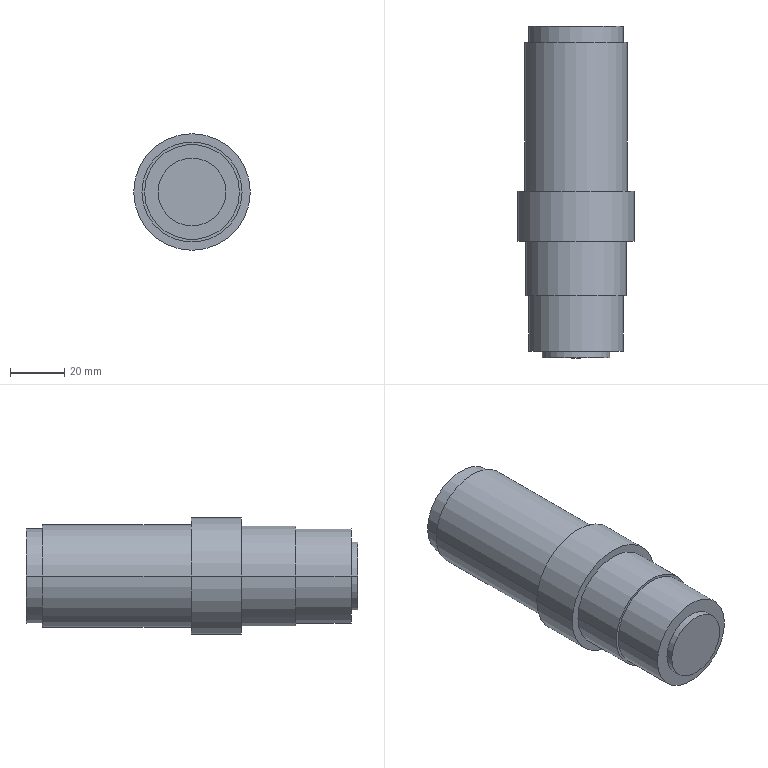Part | SolidWorks | features BaseBody 1 | 1 solid | 32 faces | box 43 x 122.5 x 43 mm | volume 103084 mm3 | cylinder 14 | plane 12 | cone 6 | commonest cylinder face diameters 35 x4 6 x2 25 x2 37 x2 38 x2 43 x2
STEP:
#1=CARTESIAN_POINT('',(-19.,59.,0.));
#2=VERTEX_POINT('',#1);
#3=CARTESIAN_POINT('',(19.,59.,0.));
#4=VERTEX_POINT('',#3);
#5=CARTESIAN_POINT('',(0.,59.,0.));
#6=DIRECTION('',(0.,1.,0.));
#7=DIRECTION('',(-1.,0.,0.));
#8=AXIS2_PLACEMENT_3D('',#5,#6,#7);
#9=CIRCLE('',#8,19.);
#10=EDGE_CURVE('',#2,#4,#9,.T.);
#11=ORIENTED_EDGE('',*,*,#10,.T.);
#12=CARTESIAN_POINT('',(19.,114.,0.));
#13=VERTEX_POINT('',#12);
#14=CARTESIAN_POINT('',(19.,86.5,0.));
#15=DIRECTION('',(0.,1.,0.));
#16=VECTOR('',#15,1000.);
#17=LINE('',#14,#16);
#18=EDGE_CURVE('',#4,#13,#17,.T.);
#19=ORIENTED_EDGE('',*,*,#18,.T.);
#20=CARTESIAN_POINT('',(-19.,114.,0.));
#21=VERTEX_POINT('',#20);
#22=CARTESIAN_POINT('',(0.,114.,0.));
#23=DIRECTION('',(0.,-1.,0.));
#24=DIRECTION('',(-1.,0.,0.));
#25=AXIS2_PLACEMENT_3D('',#22,#23,#24);
#26=CIRCLE('',#25,19.);
#27=EDGE_CURVE('',#13,#21,#26,.T.);
#28=ORIENTED_EDGE('',*,*,#27,.T.);
#29=CARTESIAN_POINT('',(-19.,86.5,0.));
#30=DIRECTION('',(0.,1.,0.));
#31=VECTOR('',#30,1000.);
#32=LINE('',#29,#31);
#33=EDGE_CURVE('',#2,#21,#32,.T.);
#34=ORIENTED_EDGE('',*,*,#33,.F.);
#35=EDGE_LOOP('',(#11,#19,#28,#34));
#36=FACE_OUTER_BOUND('',#35,.T.);
#37=CARTESIAN_POINT('',(0.,86.5,0.));
#38=DIRECTION('',(0.,1.,0.));
#39=DIRECTION('',(-1.,0.,0.));
#40=AXIS2_PLACEMENT_3D('',#37,#38,#39);
#41=CYLINDRICAL_SURFACE('',#40,19.);
#42=ADVANCED_FACE('',(#36),#41,.T.);
#43=CARTESIAN_POINT('',(-21.5,40.5,0.));
#44=VERTEX_POINT('',#43);
#45=CARTESIAN_POINT('',(21.5,40.5,0.));
#46=VERTEX_POINT('',#45);
#47=CARTESIAN_POINT('',(0.,40.5,0.));
#48=DIRECTION('',(0.,1.,0.));
#49=DIRECTION('',(-1.,0.,0.));
#50=AXIS2_PLACEMENT_3D('',#47,#48,#49);
#51=CIRCLE('',#50,21.5);
#52=EDGE_CURVE('',#44,#46,#51,.T.);
#53=ORIENTED_EDGE('',*,*,#52,.T.);
#54=CARTESIAN_POINT('',(21.5,59.,0.));
#55=VERTEX_POINT('',#54);
#56=CARTESIAN_POINT('',(21.5,49.75,0.));
#57=DIRECTION('',(0.,1.,0.));
#58=VECTOR('',#57,1000.);
#59=LINE('',#56,#58);
#60=EDGE_CURVE('',#46,#55,#59,.T.);
#61=ORIENTED_EDGE('',*,*,#60,.T.);
#62=CARTESIAN_POINT('',(-21.5,59.,0.));
#63=VERTEX_POINT('',#62);
#64=CARTESIAN_POINT('',(0.,59.,0.));
#65=DIRECTION('',(0.,1.,0.));
#66=DIRECTION('',(-1.,0.,0.));
#67=AXIS2_PLACEMENT_3D('',#64,#65,#66);
#68=CIRCLE('',#67,21.5);
#69=EDGE_CURVE('',#63,#55,#68,.T.);
#70=ORIENTED_EDGE('',*,*,#69,.F.);
#71=CARTESIAN_POINT('',(-21.5,49.75,0.));
#72=DIRECTION('',(0.,1.,0.));
#73=VECTOR('',#72,1000.);
#74=LINE('',#71,#73);
#75=EDGE_CURVE('',#44,#63,#74,.T.);
#76=ORIENTED_EDGE('',*,*,#75,.F.);
#77=EDGE_LOOP('',(#53,#61,#70,#76));
#78=FACE_OUTER_BOUND('',#77,.T.);
#79=CARTESIAN_POINT('',(0.,49.75,0.));
#80=DIRECTION('',(0.,1.,0.));
#81=DIRECTION('',(-1.,0.,0.));
#82=AXIS2_PLACEMENT_3D('',#79,#80,#81);
#83=CYLINDRICAL_SURFACE('',#82,21.5);
#84=ADVANCED_FACE('',(#78),#83,.T.);
#85=CARTESIAN_POINT('',(17.5,114.,0.));
#86=VERTEX_POINT('',#85);
#87=CARTESIAN_POINT('',(-17.5,114.,0.));
#88=VERTEX_POINT('',#87);
#89=CARTESIAN_POINT('',(0.,114.,0.));
#90=DIRECTION('',(0.,-1.,0.));
#91=DIRECTION('',(-1.,0.,0.));
#92=AXIS2_PLACEMENT_3D('',#89,#90,#91);
#93=CIRCLE('',#92,17.5);
#94=EDGE_CURVE('',#86,#88,#93,.T.);
#95=ORIENTED_EDGE('',*,*,#94,.F.);
#96=CARTESIAN_POINT('',(17.5,120.,0.));
#97=VERTEX_POINT('',#96);
#98=CARTESIAN_POINT('',(17.5,117.,0.));
#99=DIRECTION('',(0.,1.,0.));
#100=VECTOR('',#99,1000.);
#101=LINE('',#98,#100);
#102=EDGE_CURVE('',#86,#97,#101,.T.);
#103=ORIENTED_EDGE('',*,*,#102,.T.);
#104=CARTESIAN_POINT('',(-17.5,120.,0.));
#105=VERTEX_POINT('',#104);
#106=CARTESIAN_POINT('',(0.,120.,0.));
#107=DIRECTION('',(0.,-1.,0.));
#108=DIRECTION('',(-1.,0.,0.));
#109=AXIS2_PLACEMENT_3D('',#106,#107,#108);
#110=CIRCLE('',#109,17.5);
#111=EDGE_CURVE('',#97,#105,#110,.T.);
#112=ORIENTED_EDGE('',*,*,#111,.T.);
#113=CARTESIAN_POINT('',(-17.5,117.,0.));
#114=DIRECTION('',(0.,1.,0.));
#115=VECTOR('',#114,1000.);
#116=LINE('',#113,#115);
#117=EDGE_CURVE('',#88,#105,#116,.T.);
#118=ORIENTED_EDGE('',*,*,#117,.F.);
#119=EDGE_LOOP('',(#95,#103,#112,#118));
#120=FACE_OUTER_BOUND('',#119,.T.);
#121=CARTESIAN_POINT('',(0.,117.,0.));
#122=DIRECTION('',(0.,1.,0.));
#123=DIRECTION('',(-1.,0.,0.));
#124=AXIS2_PLACEMENT_3D('',#121,#122,#123);
#125=CYLINDRICAL_SURFACE('',#124,17.5);
#126=ADVANCED_FACE('',(#120),#125,.T.);
#127=CARTESIAN_POINT('',(-18.5,20.5,0.));
#128=VERTEX_POINT('',#127);
#129=CARTESIAN_POINT('',(18.5,20.5,0.));
#130=VERTEX_POINT('',#129);
#131=CARTESIAN_POINT('',(0.,20.5,0.));
#132=DIRECTION('',(0.,1.,0.));
#133=DIRECTION('',(-1.,0.,0.));
#134=AXIS2_PLACEMENT_3D('',#131,#132,#133);
#135=CIRCLE('',#134,18.5);
#136=EDGE_CURVE('',#128,#130,#135,.T.);
#137=ORIENTED_EDGE('',*,*,#136,.T.);
#138=CARTESIAN_POINT('',(18.5,40.5,0.));
#139=VERTEX_POINT('',#138);
#140=CARTESIAN_POINT('',(18.5,30.5,0.));
#141=DIRECTION('',(0.,1.,0.));
#142=VECTOR('',#141,1000.);
#143=LINE('',#140,#142);
#144=EDGE_CURVE('',#130,#139,#143,.T.);
#145=ORIENTED_EDGE('',*,*,#144,.T.);
#146=CARTESIAN_POINT('',(-18.5,40.5,0.));
#147=VERTEX_POINT('',#146);
#148=CARTESIAN_POINT('',(0.,40.5,0.));
#149=DIRECTION('',(0.,1.,0.));
#150=DIRECTION('',(-1.,0.,0.));
#151=AXIS2_PLACEMENT_3D('',#148,#149,#150);
#152=CIRCLE('',#151,18.5);
#153=EDGE_CURVE('',#147,#139,#152,.T.);
#154=ORIENTED_EDGE('',*,*,#153,.F.);
#155=CARTESIAN_POINT('',(-18.5,30.5,0.));
#156=DIRECTION('',(0.,1.,0.));
#157=VECTOR('',#156,1000.);
#158=LINE('',#155,#157);
#159=EDGE_CURVE('',#128,#147,#158,.T.);
#160=ORIENTED_EDGE('',*,*,#159,.F.);
#161=EDGE_LOOP('',(#137,#145,#154,#160));
#162=FACE_OUTER_BOUND('',#161,.T.);
#163=CARTESIAN_POINT('',(0.,30.5,0.));
#164=DIRECTION('',(0.,1.,0.));
#165=DIRECTION('',(-1.,0.,0.));
#166=AXIS2_PLACEMENT_3D('',#163,#164,#165);
#167=CYLINDRICAL_SURFACE('',#166,18.5);
#168=ADVANCED_FACE('',(#162),#167,.T.);
#169=CARTESIAN_POINT('',(10.,118.,0.));
#170=VERTEX_POINT('',#169);
#171=CARTESIAN_POINT('',(3.,118.,-9.539));
#172=VERTEX_POINT('',#171);
#173=CARTESIAN_POINT('',(0.,118.,0.));
#174=DIRECTION('',(0.,1.,0.));
#175=DIRECTION('',(0.,0.,1.));
#176=AXIS2_PLACEMENT_3D('',#173,#174,#175);
#177=CIRCLE('',#176,10.);
#178=EDGE_CURVE('',#170,#172,#177,.T.);
#179=ORIENTED_EDGE('',*,*,#178,.F.);
#180=CARTESIAN_POINT('',(11.155,120.,0.));
#181=VERTEX_POINT('',#180);
#182=CARTESIAN_POINT('',(11.155,120.,0.));
#183=DIRECTION('',(0.5,0.866,0.));
#184=VECTOR('',#183,1000.);
#185=LINE('',#182,#184);
#186=EDGE_CURVE('',#170,#181,#185,.T.);
#187=ORIENTED_EDGE('',*,*,#186,.T.);
#188=CARTESIAN_POINT('',(3.,120.,-10.744));
#189=VERTEX_POINT('',#188);
#190=CARTESIAN_POINT('',(0.,120.,0.));
#191=DIRECTION('',(0.,-1.,0.));
#192=DIRECTION('',(-1.,0.,0.));
#193=AXIS2_PLACEMENT_3D('',#190,#191,#192);
#194=CIRCLE('',#193,11.155);
#195=EDGE_CURVE('',#189,#181,#194,.T.);
#196=ORIENTED_EDGE('',*,*,#195,.F.);
#197=CARTESIAN_POINT('',(3.,118.,-9.539));
#198=CARTESIAN_POINT('',(3.,118.666,-9.942));
#199=CARTESIAN_POINT('',(3.,119.333,-10.344));
#200=CARTESIAN_POINT('',(3.,120.,-10.744));
#201=B_SPLINE_CURVE_WITH_KNOTS('',3,(#197,#198,#199,#200),.UNSPECIFIED.,.F.,.F.,(4,4),(0.,0.002335),.UNSPECIFIED.);
#202=EDGE_CURVE('',#172,#189,#201,.T.);
#203=ORIENTED_EDGE('',*,*,#202,.F.);
#204=EDGE_LOOP('',(#179,#187,#196,#203));
#205=FACE_OUTER_BOUND('',#204,.T.);
#206=CARTESIAN_POINT('',(0.,120.,0.));
#207=DIRECTION('',(0.,1.,0.));
#208=DIRECTION('',(-1.,0.,0.));
#209=AXIS2_PLACEMENT_3D('',#206,#207,#208);
#210=CONICAL_SURFACE('',#209,11.155,0.5236);
#211=ADVANCED_FACE('',(#205),#210,.F.);
#212=ORIENTED_EDGE('',*,*,#186,.F.);
#213=CARTESIAN_POINT('',(-10.,118.,0.));
#214=VERTEX_POINT('',#213);
#215=CARTESIAN_POINT('',(0.,118.,0.));
#216=DIRECTION('',(0.,1.,0.));
#217=DIRECTION('',(0.,0.,1.));
#218=AXIS2_PLACEMENT_3D('',#215,#216,#217);
#219=CIRCLE('',#218,10.);
#220=EDGE_CURVE('',#214,#170,#219,.T.);
#221=ORIENTED_EDGE('',*,*,#220,.F.);
#222=CARTESIAN_POINT('',(-11.155,120.,0.));
#223=VERTEX_POINT('',#222);
#224=CARTESIAN_POINT('',(-11.155,120.,0.));
#225=DIRECTION('',(-0.5,0.866,0.));
#226=VECTOR('',#225,1000.);
#227=LINE('',#224,#226);
#228=EDGE_CURVE('',#214,#223,#227,.T.);
#229=ORIENTED_EDGE('',*,*,#228,.T.);
#230=CARTESIAN_POINT('',(0.,120.,0.));
#231=DIRECTION('',(0.,-1.,0.));
#232=DIRECTION('',(-1.,0.,0.));
#233=AXIS2_PLACEMENT_3D('',#230,#231,#232);
#234=CIRCLE('',#233,11.155);
#235=EDGE_CURVE('',#181,#223,#234,.T.);
#236=ORIENTED_EDGE('',*,*,#235,.F.);
#237=EDGE_LOOP('',(#212,#221,#229,#236));
#238=FACE_OUTER_BOUND('',#237,.T.);
#239=CARTESIAN_POINT('',(0.,120.,0.));
#240=DIRECTION('',(0.,1.,0.));
#241=DIRECTION('',(-1.,0.,0.));
#242=AXIS2_PLACEMENT_3D('',#239,#240,#241);
#243=CONICAL_SURFACE('',#242,11.155,0.5236);
#244=ADVANCED_FACE('',(#238),#243,.F.);
#245=CARTESIAN_POINT('',(-3.,118.,-9.539));
#246=VERTEX_POINT('',#245);
#247=CARTESIAN_POINT('',(0.,118.,0.));
#248=DIRECTION('',(0.,1.,0.));
#249=DIRECTION('',(0.,0.,1.));
#250=AXIS2_PLACEMENT_3D('',#247,#248,#249);
#251=CIRCLE('',#250,10.);
#252=EDGE_CURVE('',#246,#214,#251,.T.);
#253=ORIENTED_EDGE('',*,*,#252,.T.);
#254=CARTESIAN_POINT('',(-10.01,16.,0.));
#255=VERTEX_POINT('',#254);
#256=CARTESIAN_POINT('',(-10.01,16.,0.));
#257=DIRECTION('',(-0.00009804,-1.,0.));
#258=VECTOR('',#257,1000.);
#259=LINE('',#256,#258);
#260=EDGE_CURVE('',#214,#255,#259,.T.);
#261=ORIENTED_EDGE('',*,*,#260,.T.);
#262=CARTESIAN_POINT('',(-3.,16.,-9.55));
#263=VERTEX_POINT('',#262);
#264=CARTESIAN_POINT('',(0.,16.,0.));
#265=DIRECTION('',(0.,-1.,0.));
#266=DIRECTION('',(1.,0.,0.));
#267=AXIS2_PLACEMENT_3D('',#264,#265,#266);
#268=CIRCLE('',#267,10.01);
#269=EDGE_CURVE('',#255,#263,#268,.T.);
#270=ORIENTED_EDGE('',*,*,#269,.T.);
#271=CARTESIAN_POINT('',(-3.,118.,-9.539));
#272=DIRECTION('',(0.,-1.,-0.0001028));
#273=VECTOR('',#272,1000.);
#274=LINE('',#271,#273);
#275=EDGE_CURVE('',#246,#263,#274,.T.);
#276=ORIENTED_EDGE('',*,*,#275,.F.);
#277=EDGE_LOOP('',(#253,#261,#270,#276));
#278=FACE_OUTER_BOUND('',#277,.T.);
#279=CARTESIAN_POINT('',(0.,16.,0.));
#280=DIRECTION('',(0.,-1.,0.));
#281=DIRECTION('',(1.,0.,0.));
#282=AXIS2_PLACEMENT_3D('',#279,#280,#281);
#283=CONICAL_SURFACE('',#282,10.01,0.00009804);
#284=ADVANCED_FACE('',(#278),#283,.F.);
#285=ORIENTED_EDGE('',*,*,#260,.F.);
#286=ORIENTED_EDGE('',*,*,#220,.T.);
#287=CARTESIAN_POINT('',(10.01,16.,0.));
#288=VERTEX_POINT('',#287);
#289=CARTESIAN_POINT('',(10.01,16.,0.));
#290=DIRECTION('',(0.00009804,-1.,0.));
#291=VECTOR('',#290,1000.);
#292=LINE('',#289,#291);
#293=EDGE_CURVE('',#170,#288,#292,.T.);
#294=ORIENTED_EDGE('',*,*,#293,.T.);
#295=CARTESIAN_POINT('',(0.,16.,0.));
#296=DIRECTION('',(0.,-1.,0.));
#297=DIRECTION('',(1.,0.,0.));
#298=AXIS2_PLACEMENT_3D('',#295,#296,#297);
#299=CIRCLE('',#298,10.01);
#300=EDGE_CURVE('',#288,#255,#299,.T.);
#301=ORIENTED_EDGE('',*,*,#300,.T.);
#302=EDGE_LOOP('',(#285,#286,#294,#301));
#303=FACE_OUTER_BOUND('',#302,.T.);
#304=CARTESIAN_POINT('',(0.,16.,0.));
#305=DIRECTION('',(0.,-1.,0.));
#306=DIRECTION('',(1.,0.,0.));
#307=AXIS2_PLACEMENT_3D('',#304,#305,#306);
#308=CONICAL_SURFACE('',#307,10.01,0.00009804);
#309=ADVANCED_FACE('',(#303),#308,.F.);
#310=CARTESIAN_POINT('',(-17.5,0.,0.));
#311=VERTEX_POINT('',#310);
#312=CARTESIAN_POINT('',(17.5,0.,0.));
#313=VERTEX_POINT('',#312);
#314=CARTESIAN_POINT('',(0.,0.,0.));
#315=DIRECTION('',(0.,1.,0.));
#316=DIRECTION('',(-1.,0.,0.));
#317=AXIS2_PLACEMENT_3D('',#314,#315,#316);
#318=CIRCLE('',#317,17.5);
#319=EDGE_CURVE('',#311,#313,#318,.T.);
#320=ORIENTED_EDGE('',*,*,#319,.T.);
#321=CARTESIAN_POINT('',(17.5,20.5,0.));
#322=VERTEX_POINT('',#321);
#323=CARTESIAN_POINT('',(17.5,10.25,0.));
#324=DIRECTION('',(0.,1.,0.));
#325=VECTOR('',#324,1000.);
#326=LINE('',#323,#325);
#327=EDGE_CURVE('',#313,#322,#326,.T.);
#328=ORIENTED_EDGE('',*,*,#327,.T.);
#329=CARTESIAN_POINT('',(-17.5,20.5,0.));
#330=VERTEX_POINT('',#329);
#331=CARTESIAN_POINT('',(0.,20.5,0.));
#332=DIRECTION('',(0.,1.,0.));
#333=DIRECTION('',(-1.,0.,0.));
#334=AXIS2_PLACEMENT_3D('',#331,#332,#333);
#335=CIRCLE('',#334,17.5);
#336=EDGE_CURVE('',#330,#322,#335,.T.);
#337=ORIENTED_EDGE('',*,*,#336,.F.);
#338=CARTESIAN_POINT('',(-17.5,10.25,0.));
#339=DIRECTION('',(0.,1.,0.));
#340=VECTOR('',#339,1000.);
#341=LINE('',#338,#340);
#342=EDGE_CURVE('',#311,#330,#341,.T.);
#343=ORIENTED_EDGE('',*,*,#342,.F.);
#344=EDGE_LOOP('',(#320,#328,#337,#343));
#345=FACE_OUTER_BOUND('',#344,.T.);
#346=CARTESIAN_POINT('',(0.,10.25,0.));
#347=DIRECTION('',(0.,1.,0.));
#348=DIRECTION('',(-1.,0.,0.));
#349=AXIS2_PLACEMENT_3D('',#346,#347,#348);
#350=CYLINDRICAL_SURFACE('',#349,17.5);
#351=ADVANCED_FACE('',(#345),#350,.T.);
#352=CARTESIAN_POINT('',(-3.,16.,0.));
#353=VERTEX_POINT('',#352);
#354=CARTESIAN_POINT('',(3.,16.,0.));
#355=VERTEX_POINT('',#354);
#356=CARTESIAN_POINT('',(0.,16.,0.));
#357=DIRECTION('',(0.,1.,0.));
#358=DIRECTION('',(-1.,0.,0.));
#359=AXIS2_PLACEMENT_3D('',#356,#357,#358);
#360=CIRCLE('',#359,3.);
#361=EDGE_CURVE('',#353,#355,#360,.T.);
#362=ORIENTED_EDGE('',*,*,#361,.T.);
#363=CARTESIAN_POINT('',(3.,24.,0.));
#364=VERTEX_POINT('',#363);
#365=CARTESIAN_POINT('',(3.,20.,0.));
#366=DIRECTION('',(0.,1.,0.));
#367=VECTOR('',#366,1000.);
#368=LINE('',#365,#367);
#369=EDGE_CURVE('',#355,#364,#368,.T.);
#370=ORIENTED_EDGE('',*,*,#369,.T.);
#371=CARTESIAN_POINT('',(-3.,24.,0.));
#372=VERTEX_POINT('',#371);
#373=CARTESIAN_POINT('',(0.,24.,0.));
#374=DIRECTION('',(0.,-1.,0.));
#375=DIRECTION('',(-1.,0.,0.));
#376=AXIS2_PLACEMENT_3D('',#373,#374,#375);
#377=CIRCLE('',#376,3.);
#378=EDGE_CURVE('',#364,#372,#377,.T.);
#379=ORIENTED_EDGE('',*,*,#378,.T.);
#380=CARTESIAN_POINT('',(-3.,20.,0.));
#381=DIRECTION('',(0.,1.,0.));
#382=VECTOR('',#381,1000.);
#383=LINE('',#380,#382);
#384=EDGE_CURVE('',#353,#372,#383,.T.);
#385=ORIENTED_EDGE('',*,*,#384,.F.);
#386=EDGE_LOOP('',(#362,#370,#379,#385));
#387=FACE_OUTER_BOUND('',#386,.T.);
#388=CARTESIAN_POINT('',(0.,20.,0.));
#389=DIRECTION('',(0.,1.,0.));
#390=DIRECTION('',(-1.,0.,0.));
#391=AXIS2_PLACEMENT_3D('',#388,#389,#390);
#392=CYLINDRICAL_SURFACE('',#391,3.);
#393=ADVANCED_FACE('',(#387),#392,.T.);
#394=CARTESIAN_POINT('',(-12.5,-2.5,0.));
#395=VERTEX_POINT('',#394);
#396=CARTESIAN_POINT('',(12.5,-2.5,0.));
#397=VERTEX_POINT('',#396);
#398=CARTESIAN_POINT('',(0.,-2.5,0.));
#399=DIRECTION('',(0.,1.,0.));
#400=DIRECTION('',(-1.,0.,0.));
#401=AXIS2_PLACEMENT_3D('',#398,#399,#400);
#402=CIRCLE('',#401,12.5);
#403=EDGE_CURVE('',#395,#397,#402,.T.);
#404=ORIENTED_EDGE('',*,*,#403,.T.);
#405=CARTESIAN_POINT('',(12.5,0.,0.));
#406=VERTEX_POINT('',#405);
#407=CARTESIAN_POINT('',(12.5,-1.25,0.));
#408=DIRECTION('',(0.,1.,0.));
#409=VECTOR('',#408,1000.);
#410=LINE('',#407,#409);
#411=EDGE_CURVE('',#397,#406,#410,.T.);
#412=ORIENTED_EDGE('',*,*,#411,.T.);
#413=CARTESIAN_POINT('',(-12.5,0.,0.));
#414=VERTEX_POINT('',#413);
#415=CARTESIAN_POINT('',(0.,0.,0.));
#416=DIRECTION('',(0.,1.,0.));
#417=DIRECTION('',(-1.,0.,0.));
#418=AXIS2_PLACEMENT_3D('',#415,#416,#417);
#419=CIRCLE('',#418,12.5);
#420=EDGE_CURVE('',#414,#406,#419,.T.);
#421=ORIENTED_EDGE('',*,*,#420,.F.);
#422=CARTESIAN_POINT('',(-12.5,-1.25,0.));
#423=DIRECTION('',(0.,1.,0.));
#424=VECTOR('',#423,1000.);
#425=LINE('',#422,#424);
#426=EDGE_CURVE('',#395,#414,#425,.T.);
#427=ORIENTED_EDGE('',*,*,#426,.F.);
#428=EDGE_LOOP('',(#404,#412,#421,#427));
#429=FACE_OUTER_BOUND('',#428,.T.);
#430=CARTESIAN_POINT('',(0.,-1.25,0.));
#431=DIRECTION('',(0.,1.,0.));
#432=DIRECTION('',(-1.,0.,0.));
#433=AXIS2_PLACEMENT_3D('',#430,#431,#432);
#434=CYLINDRICAL_SURFACE('',#433,12.5);
#435=ADVANCED_FACE('',(#429),#434,.T.);
#436=ORIENTED_EDGE('',*,*,#18,.F.);
#437=CARTESIAN_POINT('',(0.,59.,0.));
#438=DIRECTION('',(0.,1.,0.));
#439=DIRECTION('',(-1.,0.,0.));
#440=AXIS2_PLACEMENT_3D('',#437,#438,#439);
#441=CIRCLE('',#440,19.);
#442=EDGE_CURVE('',#4,#2,#441,.T.);
#443=ORIENTED_EDGE('',*,*,#442,.T.);
#444=ORIENTED_EDGE('',*,*,#33,.T.);
#445=CARTESIAN_POINT('',(0.,114.,0.));
#446=DIRECTION('',(0.,-1.,0.));
#447=DIRECTION('',(-1.,0.,0.));
#448=AXIS2_PLACEMENT_3D('',#445,#446,#447);
#449=CIRCLE('',#448,19.);
#450=EDGE_CURVE('',#21,#13,#449,.T.);
#451=ORIENTED_EDGE('',*,*,#450,.T.);
#452=EDGE_LOOP('',(#436,#443,#444,#451));
#453=FACE_OUTER_BOUND('',#452,.T.);
#454=CARTESIAN_POINT('',(0.,86.5,0.));
#455=DIRECTION('',(0.,1.,0.));
#456=DIRECTION('',(-1.,0.,0.));
#457=AXIS2_PLACEMENT_3D('',#454,#455,#456);
#458=CYLINDRICAL_SURFACE('',#457,19.);
#459=ADVANCED_FACE('',(#453),#458,.T.);
#460=ORIENTED_EDGE('',*,*,#69,.T.);
#461=CARTESIAN_POINT('',(0.,59.,0.));
#462=DIRECTION('',(0.,1.,0.));
#463=DIRECTION('',(-1.,0.,0.));
#464=AXIS2_PLACEMENT_3D('',#461,#462,#463);
#465=CIRCLE('',#464,21.5);
#466=EDGE_CURVE('',#55,#63,#465,.T.);
#467=ORIENTED_EDGE('',*,*,#466,.T.);
#468=EDGE_LOOP('',(#460,#467));
#469=FACE_OUTER_BOUND('',#468,.T.);
#470=ORIENTED_EDGE('',*,*,#10,.F.);
#471=ORIENTED_EDGE('',*,*,#442,.F.);
#472=EDGE_LOOP('',(#470,#471));
#473=FACE_BOUND('',#472,.T.);
#474=CARTESIAN_POINT('',(0.,59.,20.25));
#475=DIRECTION('',(0.,1.,0.));
#476=DIRECTION('',(-1.,0.,0.));
#477=AXIS2_PLACEMENT_3D('',#474,#475,#476);
#478=PLANE('',#477);
#479=ADVANCED_FACE('',(#469,#473),#478,.T.);
#480=ORIENTED_EDGE('',*,*,#450,.F.);
#481=ORIENTED_EDGE('',*,*,#27,.F.);
#482=EDGE_LOOP('',(#480,#481));
#483=FACE_OUTER_BOUND('',#482,.T.);
#484=CARTESIAN_POINT('',(0.,114.,0.));
#485=DIRECTION('',(0.,-1.,0.));
#486=DIRECTION('',(-1.,0.,0.));
#487=AXIS2_PLACEMENT_3D('',#484,#485,#486);
#488=CIRCLE('',#487,17.5);
#489=EDGE_CURVE('',#88,#86,#488,.T.);
#490=ORIENTED_EDGE('',*,*,#489,.T.);
#491=ORIENTED_EDGE('',*,*,#94,.T.);
#492=EDGE_LOOP('',(#490,#491));
#493=FACE_BOUND('',#492,.T.);
#494=CARTESIAN_POINT('',(0.,114.,18.25));
#495=DIRECTION('',(0.,1.,0.));
#496=DIRECTION('',(-1.,0.,0.));
#497=AXIS2_PLACEMENT_3D('',#494,#495,#496);
#498=PLANE('',#497);
#499=ADVANCED_FACE('',(#483,#493),#498,.T.);
#500=ORIENTED_EDGE('',*,*,#60,.F.);
#501=CARTESIAN_POINT('',(0.,40.5,0.));
#502=DIRECTION('',(0.,1.,0.));
#503=DIRECTION('',(-1.,0.,0.));
#504=AXIS2_PLACEMENT_3D('',#501,#502,#503);
#505=CIRCLE('',#504,21.5);
#506=EDGE_CURVE('',#46,#44,#505,.T.);
#507=ORIENTED_EDGE('',*,*,#506,.T.);
#508=ORIENTED_EDGE('',*,*,#75,.T.);
#509=ORIENTED_EDGE('',*,*,#466,.F.);
#510=EDGE_LOOP('',(#500,#507,#508,#509));
#511=FACE_OUTER_BOUND('',#510,.T.);
#512=CARTESIAN_POINT('',(0.,49.75,0.));
#513=DIRECTION('',(0.,1.,0.));
#514=DIRECTION('',(-1.,0.,0.));
#515=AXIS2_PLACEMENT_3D('',#512,#513,#514);
#516=CYLINDRICAL_SURFACE('',#515,21.5);
#517=ADVANCED_FACE('',(#511),#516,.T.);
#518=ORIENTED_EDGE('',*,*,#102,.F.);
#519=ORIENTED_EDGE('',*,*,#489,.F.);
#520=ORIENTED_EDGE('',*,*,#117,.T.);
#521=CARTESIAN_POINT('',(0.,120.,0.));
#522=DIRECTION('',(0.,-1.,0.));
#523=DIRECTION('',(-1.,0.,0.));
#524=AXIS2_PLACEMENT_3D('',#521,#522,#523);
#525=CIRCLE('',#524,17.5);
#526=EDGE_CURVE('',#105,#97,#525,.T.);
#527=ORIENTED_EDGE('',*,*,#526,.T.);
#528=EDGE_LOOP('',(#518,#519,#520,#527));
#529=FACE_OUTER_BOUND('',#528,.T.);
#530=CARTESIAN_POINT('',(0.,117.,0.));
#531=DIRECTION('',(0.,1.,0.));
#532=DIRECTION('',(-1.,0.,0.));
#533=AXIS2_PLACEMENT_3D('',#530,#531,#532);
#534=CYLINDRICAL_SURFACE('',#533,17.5);
#535=ADVANCED_FACE('',(#529),#534,.T.);
#536=ORIENTED_EDGE('',*,*,#153,.T.);
#537=CARTESIAN_POINT('',(0.,40.5,0.));
#538=DIRECTION('',(0.,1.,0.));
#539=DIRECTION('',(-1.,0.,0.));
#540=AXIS2_PLACEMENT_3D('',#537,#538,#539);
#541=CIRCLE('',#540,18.5);
#542=EDGE_CURVE('',#139,#147,#541,.T.);
#543=ORIENTED_EDGE('',*,*,#542,.T.);
#544=EDGE_LOOP('',(#536,#543));
#545=FACE_BOUND('',#544,.T.);
#546=ORIENTED_EDGE('',*,*,#52,.F.);
#547=ORIENTED_EDGE('',*,*,#506,.F.);
#548=EDGE_LOOP('',(#546,#547));
#549=FACE_OUTER_BOUND('',#548,.T.);
#550=CARTESIAN_POINT('',(0.,40.5,20.));
#551=DIRECTION('',(0.,-1.,0.));
#552=DIRECTION('',(1.,0.,0.));
#553=AXIS2_PLACEMENT_3D('',#550,#551,#552);
#554=PLANE('',#553);
#555=ADVANCED_FACE('',(#545,#549),#554,.T.);
#556=ORIENTED_EDGE('',*,*,#526,.F.);
#557=ORIENTED_EDGE('',*,*,#111,.F.);
#558=EDGE_LOOP('',(#556,#557));
#559=FACE_OUTER_BOUND('',#558,.T.);
#560=CARTESIAN_POINT('',(-3.,120.,-10.744));
#561=VERTEX_POINT('',#560);
#562=CARTESIAN_POINT('',(-3.,120.,-12.8));
#563=VERTEX_POINT('',#562);
#564=CARTESIAN_POINT('',(-3.,120.,8.75));
#565=DIRECTION('',(0.,0.,-1.));
#566=VECTOR('',#565,1000.);
#567=LINE('',#564,#566);
#568=EDGE_CURVE('',#561,#563,#567,.T.);
#569=ORIENTED_EDGE('',*,*,#568,.T.);
#570=CARTESIAN_POINT('',(3.,120.,-12.8));
#571=VERTEX_POINT('',#570);
#572=CARTESIAN_POINT('',(0.,120.,-12.8));
#573=DIRECTION('',(1.,0.,0.));
#574=VECTOR('',#573,1000.);
#575=LINE('',#572,#574);
#576=EDGE_CURVE('',#563,#571,#575,.T.);
#577=ORIENTED_EDGE('',*,*,#576,.T.);
#578=CARTESIAN_POINT('',(3.,120.,8.75));
#579=DIRECTION('',(0.,0.,1.));
#580=VECTOR('',#579,1000.);
#581=LINE('',#578,#580);
#582=EDGE_CURVE('',#571,#189,#581,.T.);
#583=ORIENTED_EDGE('',*,*,#582,.T.);
#584=ORIENTED_EDGE('',*,*,#195,.T.);
#585=ORIENTED_EDGE('',*,*,#235,.T.);
#586=CARTESIAN_POINT('',(0.,120.,0.));
#587=DIRECTION('',(0.,-1.,0.));
#588=DIRECTION('',(-1.,0.,0.));
#589=AXIS2_PLACEMENT_3D('',#586,#587,#588);
#590=CIRCLE('',#589,11.155);
#591=EDGE_CURVE('',#223,#561,#590,.T.);
#592=ORIENTED_EDGE('',*,*,#591,.T.);
#593=EDGE_LOOP('',(#569,#577,#583,#584,#585,#592));
#594=FACE_BOUND('',#593,.T.);
#595=CARTESIAN_POINT('',(0.,120.,8.75));
#596=DIRECTION('',(0.,1.,0.));
#597=DIRECTION('',(-1.,0.,0.));
#598=AXIS2_PLACEMENT_3D('',#595,#596,#597);
#599=PLANE('',#598);
#600=ADVANCED_FACE('',(#559,#594),#599,.T.);
#601=ORIENTED_EDGE('',*,*,#144,.F.);
#602=CARTESIAN_POINT('',(0.,20.5,0.));
#603=DIRECTION('',(0.,1.,0.));
#604=DIRECTION('',(-1.,0.,0.));
#605=AXIS2_PLACEMENT_3D('',#602,#603,#604);
#606=CIRCLE('',#605,18.5);
#607=EDGE_CURVE('',#130,#128,#606,.T.);
#608=ORIENTED_EDGE('',*,*,#607,.T.);
#609=ORIENTED_EDGE('',*,*,#159,.T.);
#610=ORIENTED_EDGE('',*,*,#542,.F.);
#611=EDGE_LOOP('',(#601,#608,#609,#610));
#612=FACE_OUTER_BOUND('',#611,.T.);
#613=CARTESIAN_POINT('',(0.,30.5,0.));
#614=DIRECTION('',(0.,1.,0.));
#615=DIRECTION('',(-1.,0.,0.));
#616=AXIS2_PLACEMENT_3D('',#613,#614,#615);
#617=CYLINDRICAL_SURFACE('',#616,18.5);
#618=ADVANCED_FACE('',(#612),#617,.T.);
#619=ORIENTED_EDGE('',*,*,#576,.F.);
#620=CARTESIAN_POINT('',(-3.,16.,-12.8));
#621=VERTEX_POINT('',#620);
#622=CARTESIAN_POINT('',(-3.,68.,-12.8));
#623=DIRECTION('',(0.,-1.,0.));
#624=VECTOR('',#623,1000.);
#625=LINE('',#622,#624);
#626=EDGE_CURVE('',#563,#621,#625,.T.);
#627=ORIENTED_EDGE('',*,*,#626,.T.);
#628=CARTESIAN_POINT('',(3.,16.,-12.8));
#629=VERTEX_POINT('',#628);
#630=CARTESIAN_POINT('',(0.,16.,-12.8));
#631=DIRECTION('',(1.,0.,0.));
#632=VECTOR('',#631,1000.);
#633=LINE('',#630,#632);
#634=EDGE_CURVE('',#621,#629,#633,.T.);
#635=ORIENTED_EDGE('',*,*,#634,.T.);
#636=CARTESIAN_POINT('',(3.,68.,-12.8));
#637=DIRECTION('',(0.,1.,0.));
#638=VECTOR('',#637,1000.);
#639=LINE('',#636,#638);
#640=EDGE_CURVE('',#629,#571,#639,.T.);
#641=ORIENTED_EDGE('',*,*,#640,.T.);
#642=EDGE_LOOP('',(#619,#627,#635,#641));
#643=FACE_OUTER_BOUND('',#642,.T.);
#644=CARTESIAN_POINT('',(0.,68.,-12.8));
#645=DIRECTION('',(0.,0.,1.));
#646=DIRECTION('',(1.,0.,0.));
#647=AXIS2_PLACEMENT_3D('',#644,#645,#646);
#648=PLANE('',#647);
#649=ADVANCED_FACE('',(#643),#648,.T.);
#650=ORIENTED_EDGE('',*,*,#568,.F.);
#651=CARTESIAN_POINT('',(-3.,120.,-10.744));
#652=CARTESIAN_POINT('',(-3.,119.333,-10.344));
#653=CARTESIAN_POINT('',(-3.,118.666,-9.942));
#654=CARTESIAN_POINT('',(-3.,118.,-9.539));
#655=B_SPLINE_CURVE_WITH_KNOTS('',3,(#651,#652,#653,#654),.UNSPECIFIED.,.F.,.F.,(4,4),(0.,0.002335),.UNSPECIFIED.);
#656=EDGE_CURVE('',#561,#246,#655,.T.);
#657=ORIENTED_EDGE('',*,*,#656,.T.);
#658=ORIENTED_EDGE('',*,*,#275,.T.);
#659=CARTESIAN_POINT('',(-3.,16.,-9.4));
#660=DIRECTION('',(0.,0.,-1.));
#661=VECTOR('',#660,1000.);
#662=LINE('',#659,#661);
#663=EDGE_CURVE('',#263,#621,#662,.T.);
#664=ORIENTED_EDGE('',*,*,#663,.T.);
#665=ORIENTED_EDGE('',*,*,#626,.F.);
#666=EDGE_LOOP('',(#650,#657,#658,#664,#665));
#667=FACE_OUTER_BOUND('',#666,.T.);
#668=CARTESIAN_POINT('',(-3.,68.,-9.4));
#669=DIRECTION('',(1.,0.,0.));
#670=DIRECTION('',(0.,0.,-1.));
#671=AXIS2_PLACEMENT_3D('',#668,#669,#670);
#672=PLANE('',#671);
#673=ADVANCED_FACE('',(#667),#672,.T.);
#674=ORIENTED_EDGE('',*,*,#228,.F.);
#675=ORIENTED_EDGE('',*,*,#252,.F.);
#676=ORIENTED_EDGE('',*,*,#656,.F.);
#677=ORIENTED_EDGE('',*,*,#591,.F.);
#678=EDGE_LOOP('',(#674,#675,#676,#677));
#679=FACE_OUTER_BOUND('',#678,.T.);
#680=CARTESIAN_POINT('',(0.,120.,0.));
#681=DIRECTION('',(0.,1.,0.));
#682=DIRECTION('',(-1.,0.,0.));
#683=AXIS2_PLACEMENT_3D('',#680,#681,#682);
#684=CONICAL_SURFACE('',#683,11.155,0.5236);
#685=ADVANCED_FACE('',(#679),#684,.F.);
#686=ORIENTED_EDGE('',*,*,#640,.F.);
#687=CARTESIAN_POINT('',(3.,16.,-9.55));
#688=VERTEX_POINT('',#687);
#689=CARTESIAN_POINT('',(3.,16.,-9.4));
#690=DIRECTION('',(0.,0.,1.));
#691=VECTOR('',#690,1000.);
#692=LINE('',#689,#691);
#693=EDGE_CURVE('',#629,#688,#692,.T.);
#694=ORIENTED_EDGE('',*,*,#693,.T.);
#695=CARTESIAN_POINT('',(3.,16.,-9.55));
#696=DIRECTION('',(0.,1.,0.0001028));
#697=VECTOR('',#696,1000.);
#698=LINE('',#695,#697);
#699=EDGE_CURVE('',#688,#172,#698,.T.);
#700=ORIENTED_EDGE('',*,*,#699,.T.);
#701=ORIENTED_EDGE('',*,*,#202,.T.);
#702=ORIENTED_EDGE('',*,*,#582,.F.);
#703=EDGE_LOOP('',(#686,#694,#700,#701,#702));
#704=FACE_OUTER_BOUND('',#703,.T.);
#705=CARTESIAN_POINT('',(3.,68.,-9.4));
#706=DIRECTION('',(-1.,0.,0.));
#707=DIRECTION('',(0.,0.,1.));
#708=AXIS2_PLACEMENT_3D('',#705,#706,#707);
#709=PLANE('',#708);
#710=ADVANCED_FACE('',(#704),#709,.T.);
#711=ORIENTED_EDGE('',*,*,#336,.T.);
#712=CARTESIAN_POINT('',(0.,20.5,0.));
#713=DIRECTION('',(0.,1.,0.));
#714=DIRECTION('',(-1.,0.,0.));
#715=AXIS2_PLACEMENT_3D('',#712,#713,#714);
#716=CIRCLE('',#715,17.5);
#717=EDGE_CURVE('',#322,#330,#716,.T.);
#718=ORIENTED_EDGE('',*,*,#717,.T.);
#719=EDGE_LOOP('',(#711,#718));
#720=FACE_BOUND('',#719,.T.);
#721=ORIENTED_EDGE('',*,*,#136,.F.);
#722=ORIENTED_EDGE('',*,*,#607,.F.);
#723=EDGE_LOOP('',(#721,#722));
#724=FACE_OUTER_BOUND('',#723,.T.);
#725=CARTESIAN_POINT('',(0.,20.5,18.));
#726=DIRECTION('',(0.,-1.,0.));
#727=DIRECTION('',(1.,0.,0.));
#728=AXIS2_PLACEMENT_3D('',#725,#726,#727);
#729=PLANE('',#728);
#730=ADVANCED_FACE('',(#720,#724),#729,.T.);
#731=CARTESIAN_POINT('',(0.,16.,0.));
#732=DIRECTION('',(0.,-1.,0.));
#733=DIRECTION('',(1.,0.,0.));
#734=AXIS2_PLACEMENT_3D('',#731,#732,#733);
#735=CIRCLE('',#734,10.01);
#736=EDGE_CURVE('',#688,#288,#735,.T.);
#737=ORIENTED_EDGE('',*,*,#736,.F.);
#738=ORIENTED_EDGE('',*,*,#693,.F.);
#739=ORIENTED_EDGE('',*,*,#634,.F.);
#740=ORIENTED_EDGE('',*,*,#663,.F.);
#741=ORIENTED_EDGE('',*,*,#269,.F.);
#742=ORIENTED_EDGE('',*,*,#300,.F.);
#743=EDGE_LOOP('',(#737,#738,#739,#740,#741,#742));
#744=FACE_OUTER_BOUND('',#743,.T.);
#745=ORIENTED_EDGE('',*,*,#361,.F.);
#746=CARTESIAN_POINT('',(0.,16.,0.));
#747=DIRECTION('',(0.,1.,0.));
#748=DIRECTION('',(-1.,0.,0.));
#749=AXIS2_PLACEMENT_3D('',#746,#747,#748);
#750=CIRCLE('',#749,3.);
#751=EDGE_CURVE('',#355,#353,#750,.T.);
#752=ORIENTED_EDGE('',*,*,#751,.F.);
#753=EDGE_LOOP('',(#745,#752));
#754=FACE_BOUND('',#753,.T.);
#755=CARTESIAN_POINT('',(0.,16.,6.505));
#756=DIRECTION('',(0.,-1.,0.));
#757=DIRECTION('',(1.,0.,0.));
#758=AXIS2_PLACEMENT_3D('',#755,#756,#757);
#759=PLANE('',#758);
#760=ADVANCED_FACE('',(#744,#754),#759,.F.);
#761=ORIENTED_EDGE('',*,*,#293,.F.);
#762=ORIENTED_EDGE('',*,*,#178,.T.);
#763=ORIENTED_EDGE('',*,*,#699,.F.);
#764=ORIENTED_EDGE('',*,*,#736,.T.);
#765=EDGE_LOOP('',(#761,#762,#763,#764));
#766=FACE_OUTER_BOUND('',#765,.T.);
#767=CARTESIAN_POINT('',(0.,16.,0.));
#768=DIRECTION('',(0.,-1.,0.));
#769=DIRECTION('',(1.,0.,0.));
#770=AXIS2_PLACEMENT_3D('',#767,#768,#769);
#771=CONICAL_SURFACE('',#770,10.01,0.00009804);
#772=ADVANCED_FACE('',(#766),#771,.F.);
#773=ORIENTED_EDGE('',*,*,#327,.F.);
#774=CARTESIAN_POINT('',(0.,0.,0.));
#775=DIRECTION('',(0.,1.,0.));
#776=DIRECTION('',(-1.,0.,0.));
#777=AXIS2_PLACEMENT_3D('',#774,#775,#776);
#778=CIRCLE('',#777,17.5);
#779=EDGE_CURVE('',#313,#311,#778,.T.);
#780=ORIENTED_EDGE('',*,*,#779,.T.);
#781=ORIENTED_EDGE('',*,*,#342,.T.);
#782=ORIENTED_EDGE('',*,*,#717,.F.);
#783=EDGE_LOOP('',(#773,#780,#781,#782));
#784=FACE_OUTER_BOUND('',#783,.T.);
#785=CARTESIAN_POINT('',(0.,10.25,0.));
#786=DIRECTION('',(0.,1.,0.));
#787=DIRECTION('',(-1.,0.,0.));
#788=AXIS2_PLACEMENT_3D('',#785,#786,#787);
#789=CYLINDRICAL_SURFACE('',#788,17.5);
#790=ADVANCED_FACE('',(#784),#789,.T.);
#791=ORIENTED_EDGE('',*,*,#369,.F.);
#792=ORIENTED_EDGE('',*,*,#751,.T.);
#793=ORIENTED_EDGE('',*,*,#384,.T.);
#794=CARTESIAN_POINT('',(0.,24.,0.));
#795=DIRECTION('',(0.,-1.,0.));
#796=DIRECTION('',(-1.,0.,0.));
#797=AXIS2_PLACEMENT_3D('',#794,#795,#796);
#798=CIRCLE('',#797,3.);
#799=EDGE_CURVE('',#372,#364,#798,.T.);
#800=ORIENTED_EDGE('',*,*,#799,.T.);
#801=EDGE_LOOP('',(#791,#792,#793,#800));
#802=FACE_OUTER_BOUND('',#801,.T.);
#803=CARTESIAN_POINT('',(0.,20.,0.));
#804=DIRECTION('',(0.,1.,0.));
#805=DIRECTION('',(-1.,0.,0.));
#806=AXIS2_PLACEMENT_3D('',#803,#804,#805);
#807=CYLINDRICAL_SURFACE('',#806,3.);
#808=ADVANCED_FACE('',(#802),#807,.T.);
#809=ORIENTED_EDGE('',*,*,#420,.T.);
#810=CARTESIAN_POINT('',(0.,0.,0.));
#811=DIRECTION('',(0.,1.,0.));
#812=DIRECTION('',(-1.,0.,0.));
#813=AXIS2_PLACEMENT_3D('',#810,#811,#812);
#814=CIRCLE('',#813,12.5);
#815=EDGE_CURVE('',#406,#414,#814,.T.);
#816=ORIENTED_EDGE('',*,*,#815,.T.);
#817=EDGE_LOOP('',(#809,#816));
#818=FACE_BOUND('',#817,.T.);
#819=ORIENTED_EDGE('',*,*,#319,.F.);
#820=ORIENTED_EDGE('',*,*,#779,.F.);
#821=EDGE_LOOP('',(#819,#820));
#822=FACE_OUTER_BOUND('',#821,.T.);
#823=CARTESIAN_POINT('',(0.,0.,15.));
#824=DIRECTION('',(0.,-1.,0.));
#825=DIRECTION('',(1.,0.,0.));
#826=AXIS2_PLACEMENT_3D('',#823,#824,#825);
#827=PLANE('',#826);
#828=ADVANCED_FACE('',(#818,#822),#827,.T.);
#829=ORIENTED_EDGE('',*,*,#799,.F.);
#830=ORIENTED_EDGE('',*,*,#378,.F.);
#831=EDGE_LOOP('',(#829,#830));
#832=FACE_OUTER_BOUND('',#831,.T.);
#833=CARTESIAN_POINT('',(0.,24.,1.5));
#834=DIRECTION('',(0.,-1.,0.));
#835=DIRECTION('',(1.,0.,0.));
#836=AXIS2_PLACEMENT_3D('',#833,#834,#835);
#837=PLANE('',#836);
#838=ADVANCED_FACE('',(#832),#837,.F.);
#839=ORIENTED_EDGE('',*,*,#411,.F.);
#840=CARTESIAN_POINT('',(0.,-2.5,0.));
#841=DIRECTION('',(0.,1.,0.));
#842=DIRECTION('',(-1.,0.,0.));
#843=AXIS2_PLACEMENT_3D('',#840,#841,#842);
#844=CIRCLE('',#843,12.5);
#845=EDGE_CURVE('',#397,#395,#844,.T.);
#846=ORIENTED_EDGE('',*,*,#845,.T.);
#847=ORIENTED_EDGE('',*,*,#426,.T.);
#848=ORIENTED_EDGE('',*,*,#815,.F.);
#849=EDGE_LOOP('',(#839,#846,#847,#848));
#850=FACE_OUTER_BOUND('',#849,.T.);
#851=CARTESIAN_POINT('',(0.,-1.25,0.));
#852=DIRECTION('',(0.,1.,0.));
#853=DIRECTION('',(-1.,0.,0.));
#854=AXIS2_PLACEMENT_3D('',#851,#852,#853);
#855=CYLINDRICAL_SURFACE('',#854,12.5);
#856=ADVANCED_FACE('',(#850),#855,.T.);
#857=ORIENTED_EDGE('',*,*,#403,.F.);
#858=ORIENTED_EDGE('',*,*,#845,.F.);
#859=EDGE_LOOP('',(#857,#858));
#860=FACE_OUTER_BOUND('',#859,.T.);
#861=CARTESIAN_POINT('',(0.,-2.5,6.25));
#862=DIRECTION('',(0.,-1.,0.));
#863=DIRECTION('',(1.,0.,0.));
#864=AXIS2_PLACEMENT_3D('',#861,#862,#863);
#865=PLANE('',#864);
#866=ADVANCED_FACE('',(#860),#865,.T.);
#867=CLOSED_SHELL('',(#42,#84,#126,#168,#211,#244,#284,#309,#351,#393,#435,#459,#479,#499,#517,#535,#555,#600,#618,#649,#673,#685,#710,#730,#760,#772,#790,#808,#828,#838,#856,#866));
#868=MANIFOLD_SOLID_BREP('',#867);
#869=CARTESIAN_POINT('',(0.,0.,0.));
#870=DIRECTION('',(0.,0.,1.));
#871=DIRECTION('',(1.,0.,0.));
#872=AXIS2_PLACEMENT_3D('',#869,#870,#871);
#873=(LENGTH_UNIT()NAMED_UNIT(*)SI_UNIT(.MILLI.,.METRE.));
#874=UNCERTAINTY_MEASURE_WITH_UNIT(LENGTH_MEASURE(0.00001),#873,'','');
#875=(NAMED_UNIT(*)PLANE_ANGLE_UNIT()SI_UNIT($,.RADIAN.));
#876=(NAMED_UNIT(*)SI_UNIT($,.STERADIAN.)SOLID_ANGLE_UNIT());
#877=(GEOMETRIC_REPRESENTATION_CONTEXT(3)GLOBAL_UNCERTAINTY_ASSIGNED_CONTEXT((#874))GLOBAL_UNIT_ASSIGNED_CONTEXT((#873,#875,#876))REPRESENTATION_CONTEXT('',''));
#878=ADVANCED_BREP_SHAPE_REPRESENTATION('',(#868,#872),#877);